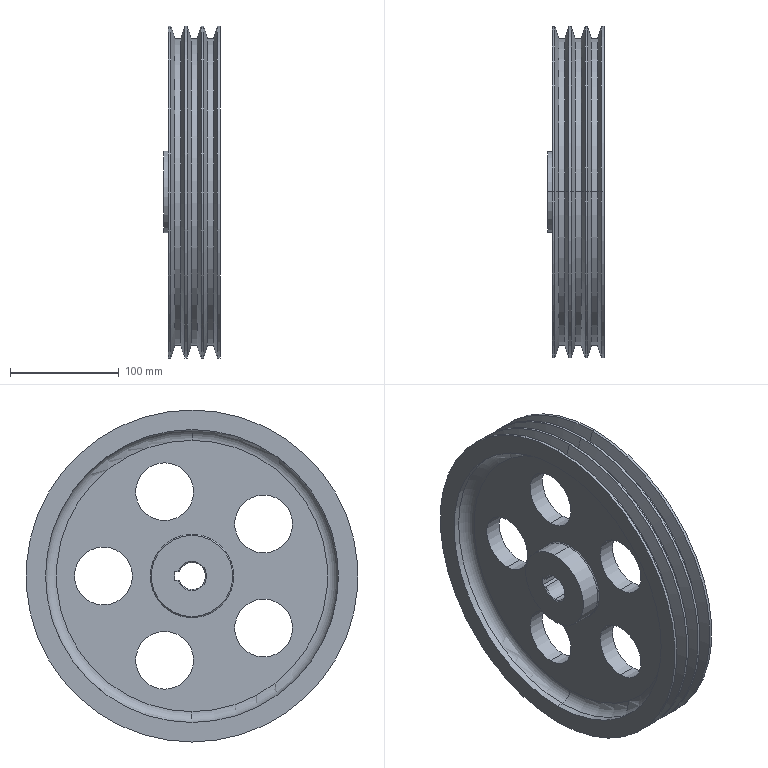Part | SolidWorks | features ICE 6, Chamfer 2, CirPattern 1, Fillet 1, Revolution 1 | 1 solid | 70 faces | box 52 x 306 x 306 mm | volume 1368961 mm3 | cylinder 35 | cone 22 | plane 9 | torus 4 | commonest cylinder face diameters 53.3 x10 306 x8 283 x6 75 x4 270 x4 25 x3